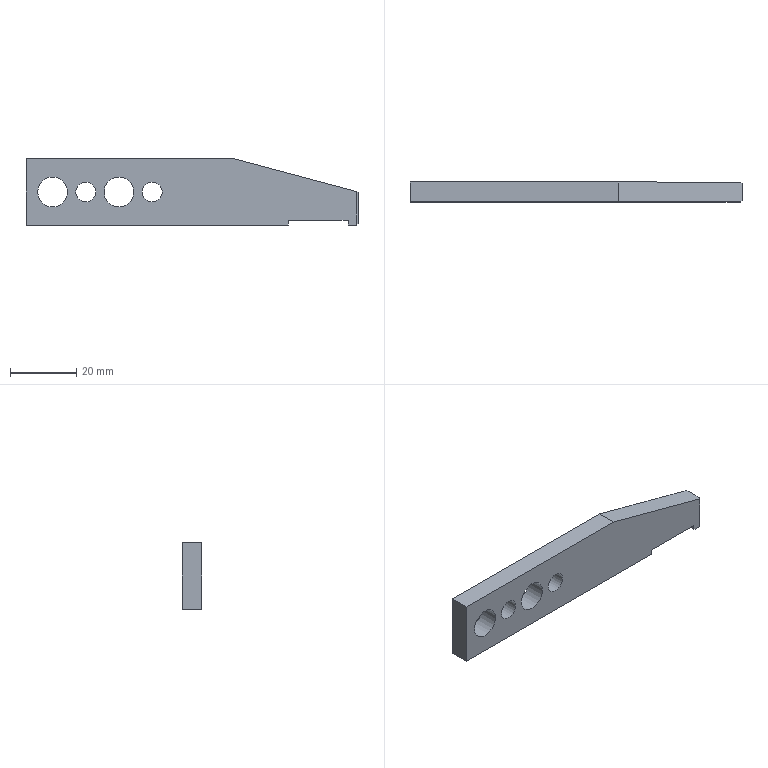Part | NX | features BREP 1 | 1 solid | 18 faces | box 100 x 6 x 20 mm | volume 9606 mm3 | plane 12 | cylinder 6 | commonest cylinder face diameters 6 x2 9 x2 19 x2
STEP:
#1=CARTESIAN_POINT('',(-21.014,3.,0.));
#2=VERTEX_POINT('',#1);
#3=CARTESIAN_POINT('',(-100.,3.,0.));
#4=VERTEX_POINT('',#3);
#5=CARTESIAN_POINT('',(-100.,3.,0.));
#6=DIRECTION('',(-1.,0.,0.));
#7=VECTOR('',#6,1000.);
#8=LINE('',#5,#7);
#9=EDGE_CURVE('',#2,#4,#8,.T.);
#10=ORIENTED_EDGE('',*,*,#9,.F.);
#11=CARTESIAN_POINT('',(-21.014,-3.,0.));
#12=VERTEX_POINT('',#11);
#13=CARTESIAN_POINT('',(-12.,0.,0.));
#14=DIRECTION('',(0.,0.,-1.));
#15=DIRECTION('',(-1.,0.,0.));
#16=AXIS2_PLACEMENT_3D('',#13,#14,#15);
#17=CIRCLE('',#16,9.5);
#18=EDGE_CURVE('',#12,#2,#17,.T.);
#19=ORIENTED_EDGE('',*,*,#18,.F.);
#20=CARTESIAN_POINT('',(-100.,-3.,0.));
#21=VERTEX_POINT('',#20);
#22=CARTESIAN_POINT('',(-100.,-3.,0.));
#23=DIRECTION('',(-1.,0.,0.));
#24=VECTOR('',#23,1000.);
#25=LINE('',#22,#24);
#26=EDGE_CURVE('',#12,#21,#25,.T.);
#27=ORIENTED_EDGE('',*,*,#26,.T.);
#28=CARTESIAN_POINT('',(-100.,3.,0.));
#29=DIRECTION('',(0.,-1.,0.));
#30=VECTOR('',#29,1000.);
#31=LINE('',#28,#30);
#32=EDGE_CURVE('',#4,#21,#31,.T.);
#33=ORIENTED_EDGE('',*,*,#32,.F.);
#34=EDGE_LOOP('',(#10,#19,#27,#33));
#35=FACE_BOUND('',#34,.T.);
#36=CARTESIAN_POINT('',(-100.,3.,0.));
#37=DIRECTION('',(0.,0.,1.));
#38=DIRECTION('',(-1.,0.,0.));
#39=AXIS2_PLACEMENT_3D('',#36,#37,#38);
#40=PLANE('',#39);
#41=ADVANCED_FACE('',(#35),#40,.F.);
#42=CARTESIAN_POINT('',(-100.,-3.,20.));
#43=VERTEX_POINT('',#42);
#44=CARTESIAN_POINT('',(-100.,-3.,25.));
#45=DIRECTION('',(0.,0.,1.));
#46=VECTOR('',#45,1000.);
#47=LINE('',#44,#46);
#48=EDGE_CURVE('',#21,#43,#47,.T.);
#49=ORIENTED_EDGE('',*,*,#48,.T.);
#50=CARTESIAN_POINT('',(-100.,3.,20.));
#51=VERTEX_POINT('',#50);
#52=CARTESIAN_POINT('',(-100.,-65.879,20.));
#53=DIRECTION('',(0.,1.,0.));
#54=VECTOR('',#53,1000.);
#55=LINE('',#52,#54);
#56=EDGE_CURVE('',#43,#51,#55,.T.);
#57=ORIENTED_EDGE('',*,*,#56,.T.);
#58=CARTESIAN_POINT('',(-100.,3.,25.));
#59=DIRECTION('',(0.,0.,1.));
#60=VECTOR('',#59,1000.);
#61=LINE('',#58,#60);
#62=EDGE_CURVE('',#4,#51,#61,.T.);
#63=ORIENTED_EDGE('',*,*,#62,.F.);
#64=ORIENTED_EDGE('',*,*,#32,.T.);
#65=EDGE_LOOP('',(#49,#57,#63,#64));
#66=FACE_BOUND('',#65,.T.);
#67=CARTESIAN_POINT('',(-100.,3.,25.));
#68=DIRECTION('',(1.,0.,0.));
#69=DIRECTION('',(0.,0.,1.));
#70=AXIS2_PLACEMENT_3D('',#67,#68,#69);
#71=PLANE('',#70);
#72=ADVANCED_FACE('',(#66),#71,.F.);
#73=CARTESIAN_POINT('',(-37.321,3.,20.));
#74=VERTEX_POINT('',#73);
#75=CARTESIAN_POINT('',(-0.5,3.,10.134));
#76=VERTEX_POINT('',#75);
#77=CARTESIAN_POINT('',(0.,3.,10.));
#78=DIRECTION('',(0.9659,0.,-0.2588));
#79=VECTOR('',#78,1000.);
#80=LINE('',#77,#79);
#81=EDGE_CURVE('',#74,#76,#80,.T.);
#82=ORIENTED_EDGE('',*,*,#81,.F.);
#83=CARTESIAN_POINT('',(-37.321,-3.,20.));
#84=VERTEX_POINT('',#83);
#85=CARTESIAN_POINT('',(-37.321,-65.879,20.));
#86=DIRECTION('',(0.,1.,0.));
#87=VECTOR('',#86,1000.);
#88=LINE('',#85,#87);
#89=EDGE_CURVE('',#84,#74,#88,.T.);
#90=ORIENTED_EDGE('',*,*,#89,.F.);
#91=CARTESIAN_POINT('',(-0.5,-3.,10.134));
#92=VERTEX_POINT('',#91);
#93=CARTESIAN_POINT('',(0.,-3.,10.));
#94=DIRECTION('',(0.9659,0.,-0.2588));
#95=VECTOR('',#94,1000.);
#96=LINE('',#93,#95);
#97=EDGE_CURVE('',#84,#92,#96,.T.);
#98=ORIENTED_EDGE('',*,*,#97,.T.);
#99=CARTESIAN_POINT('',(0.,-2.5,10.));
#100=VERTEX_POINT('',#99);
#101=CARTESIAN_POINT('',(1.293,-1.207,9.653));
#102=DIRECTION('',(0.6947,0.6947,-0.1862));
#103=VECTOR('',#102,1000.);
#104=LINE('',#101,#103);
#105=EDGE_CURVE('',#92,#100,#104,.T.);
#106=ORIENTED_EDGE('',*,*,#105,.T.);
#107=CARTESIAN_POINT('',(0.,2.5,10.));
#108=VERTEX_POINT('',#107);
#109=CARTESIAN_POINT('',(0.,3.,10.));
#110=DIRECTION('',(0.,-1.,0.));
#111=VECTOR('',#110,1000.);
#112=LINE('',#109,#111);
#113=EDGE_CURVE('',#108,#100,#112,.T.);
#114=ORIENTED_EDGE('',*,*,#113,.F.);
#115=CARTESIAN_POINT('',(0.8106,1.689,9.783));
#116=DIRECTION('',(-0.6947,0.6947,0.1862));
#117=VECTOR('',#116,1000.);
#118=LINE('',#115,#117);
#119=EDGE_CURVE('',#108,#76,#118,.T.);
#120=ORIENTED_EDGE('',*,*,#119,.T.);
#121=EDGE_LOOP('',(#82,#90,#98,#106,#114,#120));
#122=FACE_BOUND('',#121,.T.);
#123=CARTESIAN_POINT('',(0.,3.,10.));
#124=DIRECTION('',(-0.2588,0.,-0.9659));
#125=DIRECTION('',(0.9659,0.,-0.2588));
#126=AXIS2_PLACEMENT_3D('',#123,#124,#125);
#127=PLANE('',#126);
#128=ADVANCED_FACE('',(#122),#127,.F.);
#129=ORIENTED_EDGE('',*,*,#113,.T.);
#130=CARTESIAN_POINT('',(0.,-2.5,0.5));
#131=VERTEX_POINT('',#130);
#132=CARTESIAN_POINT('',(0.,-2.5,0.5));
#133=DIRECTION('',(0.,0.,-1.));
#134=VECTOR('',#133,1000.);
#135=LINE('',#132,#134);
#136=EDGE_CURVE('',#100,#131,#135,.T.);
#137=ORIENTED_EDGE('',*,*,#136,.T.);
#138=CARTESIAN_POINT('',(0.,2.5,0.5));
#139=VERTEX_POINT('',#138);
#140=CARTESIAN_POINT('',(0.,3.,0.5));
#141=DIRECTION('',(0.,1.,0.));
#142=VECTOR('',#141,1000.);
#143=LINE('',#140,#142);
#144=EDGE_CURVE('',#131,#139,#143,.T.);
#145=ORIENTED_EDGE('',*,*,#144,.T.);
#146=CARTESIAN_POINT('',(0.,2.5,0.));
#147=DIRECTION('',(0.,0.,1.));
#148=VECTOR('',#147,1000.);
#149=LINE('',#146,#148);
#150=EDGE_CURVE('',#139,#108,#149,.T.);
#151=ORIENTED_EDGE('',*,*,#150,.T.);
#152=EDGE_LOOP('',(#129,#137,#145,#151));
#153=FACE_BOUND('',#152,.T.);
#154=CARTESIAN_POINT('',(0.,3.,0.));
#155=DIRECTION('',(-1.,0.,0.));
#156=DIRECTION('',(0.,0.,-1.));
#157=AXIS2_PLACEMENT_3D('',#154,#155,#156);
#158=PLANE('',#157);
#159=ADVANCED_FACE('',(#153),#158,.F.);
#160=CARTESIAN_POINT('',(-0.5,3.,0.));
#161=VERTEX_POINT('',#160);
#162=CARTESIAN_POINT('',(-2.986,3.,0.));
#163=VERTEX_POINT('',#162);
#164=CARTESIAN_POINT('',(-100.,3.,0.));
#165=DIRECTION('',(-1.,0.,0.));
#166=VECTOR('',#165,1000.);
#167=LINE('',#164,#166);
#168=EDGE_CURVE('',#161,#163,#167,.T.);
#169=ORIENTED_EDGE('',*,*,#168,.F.);
#170=CARTESIAN_POINT('',(-0.5,-3.,0.));
#171=VERTEX_POINT('',#170);
#172=CARTESIAN_POINT('',(-0.5,3.,0.));
#173=DIRECTION('',(0.,-1.,0.));
#174=VECTOR('',#173,1000.);
#175=LINE('',#172,#174);
#176=EDGE_CURVE('',#161,#171,#175,.T.);
#177=ORIENTED_EDGE('',*,*,#176,.T.);
#178=CARTESIAN_POINT('',(-2.986,-3.,0.));
#179=VERTEX_POINT('',#178);
#180=CARTESIAN_POINT('',(-100.,-3.,0.));
#181=DIRECTION('',(-1.,0.,0.));
#182=VECTOR('',#181,1000.);
#183=LINE('',#180,#182);
#184=EDGE_CURVE('',#171,#179,#183,.T.);
#185=ORIENTED_EDGE('',*,*,#184,.T.);
#186=CARTESIAN_POINT('',(-12.,0.,0.));
#187=DIRECTION('',(0.,0.,-1.));
#188=DIRECTION('',(-1.,0.,0.));
#189=AXIS2_PLACEMENT_3D('',#186,#187,#188);
#190=CIRCLE('',#189,9.5);
#191=EDGE_CURVE('',#163,#179,#190,.T.);
#192=ORIENTED_EDGE('',*,*,#191,.F.);
#193=EDGE_LOOP('',(#169,#177,#185,#192));
#194=FACE_BOUND('',#193,.T.);
#195=CARTESIAN_POINT('',(-100.,3.,0.));
#196=DIRECTION('',(0.,0.,1.));
#197=DIRECTION('',(-1.,0.,0.));
#198=AXIS2_PLACEMENT_3D('',#195,#196,#197);
#199=PLANE('',#198);
#200=ADVANCED_FACE('',(#194),#199,.F.);
#201=CARTESIAN_POINT('',(-72.,3.,14.5));
#202=VERTEX_POINT('',#201);
#203=CARTESIAN_POINT('',(-72.,3.,10.));
#204=DIRECTION('',(0.,1.,0.));
#205=DIRECTION('',(0.,0.,1.));
#206=AXIS2_PLACEMENT_3D('',#203,#204,#205);
#207=CIRCLE('',#206,4.5);
#208=EDGE_CURVE('',#202,#202,#207,.T.);
#209=ORIENTED_EDGE('',*,*,#208,.F.);
#210=EDGE_LOOP('',(#209));
#211=FACE_BOUND('',#210,.T.);
#212=CARTESIAN_POINT('',(-92.,3.,14.5));
#213=VERTEX_POINT('',#212);
#214=CARTESIAN_POINT('',(-92.,3.,10.));
#215=DIRECTION('',(0.,1.,0.));
#216=DIRECTION('',(0.,0.,1.));
#217=AXIS2_PLACEMENT_3D('',#214,#215,#216);
#218=CIRCLE('',#217,4.5);
#219=EDGE_CURVE('',#213,#213,#218,.T.);
#220=ORIENTED_EDGE('',*,*,#219,.F.);
#221=EDGE_LOOP('',(#220));
#222=FACE_BOUND('',#221,.T.);
#223=CARTESIAN_POINT('',(-82.,3.,13.));
#224=VERTEX_POINT('',#223);
#225=CARTESIAN_POINT('',(-82.,3.,10.));
#226=DIRECTION('',(0.,1.,0.));
#227=DIRECTION('',(0.,0.,1.));
#228=AXIS2_PLACEMENT_3D('',#225,#226,#227);
#229=CIRCLE('',#228,3.);
#230=EDGE_CURVE('',#224,#224,#229,.T.);
#231=ORIENTED_EDGE('',*,*,#230,.F.);
#232=EDGE_LOOP('',(#231));
#233=FACE_BOUND('',#232,.T.);
#234=CARTESIAN_POINT('',(-62.,3.,13.));
#235=VERTEX_POINT('',#234);
#236=CARTESIAN_POINT('',(-62.,3.,10.));
#237=DIRECTION('',(0.,1.,0.));
#238=DIRECTION('',(0.,0.,1.));
#239=AXIS2_PLACEMENT_3D('',#236,#237,#238);
#240=CIRCLE('',#239,3.);
#241=EDGE_CURVE('',#235,#235,#240,.T.);
#242=ORIENTED_EDGE('',*,*,#241,.F.);
#243=EDGE_LOOP('',(#242));
#244=FACE_BOUND('',#243,.T.);
#245=ORIENTED_EDGE('',*,*,#62,.T.);
#246=CARTESIAN_POINT('',(-100.,3.,20.));
#247=DIRECTION('',(-1.,0.,0.));
#248=VECTOR('',#247,1000.);
#249=LINE('',#246,#248);
#250=EDGE_CURVE('',#74,#51,#249,.T.);
#251=ORIENTED_EDGE('',*,*,#250,.F.);
#252=ORIENTED_EDGE('',*,*,#81,.T.);
#253=CARTESIAN_POINT('',(-0.5,3.,0.));
#254=DIRECTION('',(0.,0.,-1.));
#255=VECTOR('',#254,1000.);
#256=LINE('',#253,#255);
#257=EDGE_CURVE('',#76,#161,#256,.T.);
#258=ORIENTED_EDGE('',*,*,#257,.T.);
#259=ORIENTED_EDGE('',*,*,#168,.T.);
#260=CARTESIAN_POINT('',(-2.986,3.,1.5));
#261=VERTEX_POINT('',#260);
#262=CARTESIAN_POINT('',(-2.986,3.,1.5));
#263=DIRECTION('',(0.,0.,1.));
#264=VECTOR('',#263,1000.);
#265=LINE('',#262,#264);
#266=EDGE_CURVE('',#163,#261,#265,.T.);
#267=ORIENTED_EDGE('',*,*,#266,.T.);
#268=CARTESIAN_POINT('',(-21.014,3.,1.5));
#269=VERTEX_POINT('',#268);
#270=CARTESIAN_POINT('',(0.,3.,1.5));
#271=DIRECTION('',(1.,0.,0.));
#272=VECTOR('',#271,1000.);
#273=LINE('',#270,#272);
#274=EDGE_CURVE('',#269,#261,#273,.T.);
#275=ORIENTED_EDGE('',*,*,#274,.F.);
#276=CARTESIAN_POINT('',(-21.014,3.,1.5));
#277=DIRECTION('',(0.,0.,-1.));
#278=VECTOR('',#277,1000.);
#279=LINE('',#276,#278);
#280=EDGE_CURVE('',#269,#2,#279,.T.);
#281=ORIENTED_EDGE('',*,*,#280,.T.);
#282=ORIENTED_EDGE('',*,*,#9,.T.);
#283=EDGE_LOOP('',(#245,#251,#252,#258,#259,#267,#275,#281,#282));
#284=FACE_BOUND('',#283,.T.);
#285=CARTESIAN_POINT('',(0.,3.,0.));
#286=DIRECTION('',(0.,-1.,0.));
#287=DIRECTION('',(0.,0.,1.));
#288=AXIS2_PLACEMENT_3D('',#285,#286,#287);
#289=PLANE('',#288);
#290=ADVANCED_FACE('',(#211,#222,#233,#244,#284),#289,.F.);
#291=CARTESIAN_POINT('',(-100.,-3.,20.));
#292=DIRECTION('',(-1.,0.,0.));
#293=VECTOR('',#292,1000.);
#294=LINE('',#291,#293);
#295=EDGE_CURVE('',#84,#43,#294,.T.);
#296=ORIENTED_EDGE('',*,*,#295,.T.);
#297=ORIENTED_EDGE('',*,*,#48,.F.);
#298=ORIENTED_EDGE('',*,*,#26,.F.);
#299=CARTESIAN_POINT('',(-21.014,-3.,1.5));
#300=VERTEX_POINT('',#299);
#301=CARTESIAN_POINT('',(-21.014,-3.,1.5));
#302=DIRECTION('',(0.,0.,-1.));
#303=VECTOR('',#302,1000.);
#304=LINE('',#301,#303);
#305=EDGE_CURVE('',#300,#12,#304,.T.);
#306=ORIENTED_EDGE('',*,*,#305,.F.);
#307=CARTESIAN_POINT('',(-2.986,-3.,1.5));
#308=VERTEX_POINT('',#307);
#309=CARTESIAN_POINT('',(0.,-3.,1.5));
#310=DIRECTION('',(1.,0.,0.));
#311=VECTOR('',#310,1000.);
#312=LINE('',#309,#311);
#313=EDGE_CURVE('',#300,#308,#312,.T.);
#314=ORIENTED_EDGE('',*,*,#313,.T.);
#315=CARTESIAN_POINT('',(-2.986,-3.,1.5));
#316=DIRECTION('',(0.,0.,1.));
#317=VECTOR('',#316,1000.);
#318=LINE('',#315,#317);
#319=EDGE_CURVE('',#179,#308,#318,.T.);
#320=ORIENTED_EDGE('',*,*,#319,.F.);
#321=ORIENTED_EDGE('',*,*,#184,.F.);
#322=CARTESIAN_POINT('',(-0.5,-3.,10.));
#323=DIRECTION('',(0.,0.,1.));
#324=VECTOR('',#323,1000.);
#325=LINE('',#322,#324);
#326=EDGE_CURVE('',#171,#92,#325,.T.);
#327=ORIENTED_EDGE('',*,*,#326,.T.);
#328=ORIENTED_EDGE('',*,*,#97,.F.);
#329=EDGE_LOOP('',(#296,#297,#298,#306,#314,#320,#321,#327,#328));
#330=FACE_BOUND('',#329,.T.);
#331=CARTESIAN_POINT('',(-72.,-3.,14.5));
#332=VERTEX_POINT('',#331);
#333=CARTESIAN_POINT('',(-72.,-3.,10.));
#334=DIRECTION('',(0.,1.,0.));
#335=DIRECTION('',(0.,0.,1.));
#336=AXIS2_PLACEMENT_3D('',#333,#334,#335);
#337=CIRCLE('',#336,4.5);
#338=EDGE_CURVE('',#332,#332,#337,.T.);
#339=ORIENTED_EDGE('',*,*,#338,.T.);
#340=EDGE_LOOP('',(#339));
#341=FACE_BOUND('',#340,.T.);
#342=CARTESIAN_POINT('',(-92.,-3.,14.5));
#343=VERTEX_POINT('',#342);
#344=CARTESIAN_POINT('',(-92.,-3.,10.));
#345=DIRECTION('',(0.,1.,0.));
#346=DIRECTION('',(0.,0.,1.));
#347=AXIS2_PLACEMENT_3D('',#344,#345,#346);
#348=CIRCLE('',#347,4.5);
#349=EDGE_CURVE('',#343,#343,#348,.T.);
#350=ORIENTED_EDGE('',*,*,#349,.T.);
#351=EDGE_LOOP('',(#350));
#352=FACE_BOUND('',#351,.T.);
#353=CARTESIAN_POINT('',(-82.,-3.,13.));
#354=VERTEX_POINT('',#353);
#355=CARTESIAN_POINT('',(-82.,-3.,10.));
#356=DIRECTION('',(0.,1.,0.));
#357=DIRECTION('',(0.,0.,1.));
#358=AXIS2_PLACEMENT_3D('',#355,#356,#357);
#359=CIRCLE('',#358,3.);
#360=EDGE_CURVE('',#354,#354,#359,.T.);
#361=ORIENTED_EDGE('',*,*,#360,.T.);
#362=EDGE_LOOP('',(#361));
#363=FACE_BOUND('',#362,.T.);
#364=CARTESIAN_POINT('',(-62.,-3.,13.));
#365=VERTEX_POINT('',#364);
#366=CARTESIAN_POINT('',(-62.,-3.,10.));
#367=DIRECTION('',(0.,1.,0.));
#368=DIRECTION('',(0.,0.,1.));
#369=AXIS2_PLACEMENT_3D('',#366,#367,#368);
#370=CIRCLE('',#369,3.);
#371=EDGE_CURVE('',#365,#365,#370,.T.);
#372=ORIENTED_EDGE('',*,*,#371,.T.);
#373=EDGE_LOOP('',(#372));
#374=FACE_BOUND('',#373,.T.);
#375=CARTESIAN_POINT('',(0.,-3.,0.));
#376=DIRECTION('',(0.,-1.,0.));
#377=DIRECTION('',(0.,0.,1.));
#378=AXIS2_PLACEMENT_3D('',#375,#376,#377);
#379=PLANE('',#378);
#380=ADVANCED_FACE('',(#330,#341,#352,#363,#374),#379,.T.);
#381=CARTESIAN_POINT('',(-12.,0.,1.5));
#382=DIRECTION('',(0.,0.,-1.));
#383=DIRECTION('',(-1.,0.,0.));
#384=AXIS2_PLACEMENT_3D('',#381,#382,#383);
#385=CIRCLE('',#384,9.5);
#386=EDGE_CURVE('',#300,#269,#385,.T.);
#387=ORIENTED_EDGE('',*,*,#386,.F.);
#388=ORIENTED_EDGE('',*,*,#305,.T.);
#389=ORIENTED_EDGE('',*,*,#18,.T.);
#390=ORIENTED_EDGE('',*,*,#280,.F.);
#391=EDGE_LOOP('',(#387,#388,#389,#390));
#392=FACE_BOUND('',#391,.T.);
#393=CARTESIAN_POINT('',(-12.,0.,1.5));
#394=DIRECTION('',(0.,0.,-1.));
#395=DIRECTION('',(1.,0.,0.));
#396=AXIS2_PLACEMENT_3D('',#393,#394,#395);
#397=CYLINDRICAL_SURFACE('',#396,9.5);
#398=ADVANCED_FACE('',(#392),#397,.F.);
#399=ORIENTED_EDGE('',*,*,#191,.T.);
#400=ORIENTED_EDGE('',*,*,#319,.T.);
#401=CARTESIAN_POINT('',(-12.,0.,1.5));
#402=DIRECTION('',(0.,0.,-1.));
#403=DIRECTION('',(-1.,0.,0.));
#404=AXIS2_PLACEMENT_3D('',#401,#402,#403);
#405=CIRCLE('',#404,9.5);
#406=EDGE_CURVE('',#261,#308,#405,.T.);
#407=ORIENTED_EDGE('',*,*,#406,.F.);
#408=ORIENTED_EDGE('',*,*,#266,.F.);
#409=EDGE_LOOP('',(#399,#400,#407,#408));
#410=FACE_BOUND('',#409,.T.);
#411=CARTESIAN_POINT('',(-12.,0.,1.5));
#412=DIRECTION('',(0.,0.,-1.));
#413=DIRECTION('',(1.,0.,0.));
#414=AXIS2_PLACEMENT_3D('',#411,#412,#413);
#415=CYLINDRICAL_SURFACE('',#414,9.5);
#416=ADVANCED_FACE('',(#410),#415,.F.);
#417=ORIENTED_EDGE('',*,*,#274,.T.);
#418=ORIENTED_EDGE('',*,*,#406,.T.);
#419=ORIENTED_EDGE('',*,*,#313,.F.);
#420=ORIENTED_EDGE('',*,*,#386,.T.);
#421=EDGE_LOOP('',(#417,#418,#419,#420));
#422=FACE_BOUND('',#421,.T.);
#423=CARTESIAN_POINT('',(-12.,0.,1.5));
#424=DIRECTION('',(0.,0.,-1.));
#425=DIRECTION('',(1.,0.,0.));
#426=AXIS2_PLACEMENT_3D('',#423,#424,#425);
#427=PLANE('',#426);
#428=ADVANCED_FACE('',(#422),#427,.T.);
#429=ORIENTED_EDGE('',*,*,#371,.F.);
#430=EDGE_LOOP('',(#429));
#431=FACE_BOUND('',#430,.T.);
#432=ORIENTED_EDGE('',*,*,#241,.T.);
#433=EDGE_LOOP('',(#432));
#434=FACE_BOUND('',#433,.T.);
#435=CARTESIAN_POINT('',(-62.,3.,10.));
#436=DIRECTION('',(0.,1.,0.));
#437=DIRECTION('',(0.,0.,-1.));
#438=AXIS2_PLACEMENT_3D('',#435,#436,#437);
#439=CYLINDRICAL_SURFACE('',#438,3.);
#440=ADVANCED_FACE('',(#431,#434),#439,.F.);
#441=ORIENTED_EDGE('',*,*,#360,.F.);
#442=EDGE_LOOP('',(#441));
#443=FACE_BOUND('',#442,.T.);
#444=ORIENTED_EDGE('',*,*,#230,.T.);
#445=EDGE_LOOP('',(#444));
#446=FACE_BOUND('',#445,.T.);
#447=CARTESIAN_POINT('',(-82.,3.,10.));
#448=DIRECTION('',(0.,1.,0.));
#449=DIRECTION('',(0.,0.,-1.));
#450=AXIS2_PLACEMENT_3D('',#447,#448,#449);
#451=CYLINDRICAL_SURFACE('',#450,3.);
#452=ADVANCED_FACE('',(#443,#446),#451,.F.);
#453=ORIENTED_EDGE('',*,*,#349,.F.);
#454=EDGE_LOOP('',(#453));
#455=FACE_BOUND('',#454,.T.);
#456=ORIENTED_EDGE('',*,*,#219,.T.);
#457=EDGE_LOOP('',(#456));
#458=FACE_BOUND('',#457,.T.);
#459=CARTESIAN_POINT('',(-92.,3.,10.));
#460=DIRECTION('',(0.,1.,0.));
#461=DIRECTION('',(0.,0.,-1.));
#462=AXIS2_PLACEMENT_3D('',#459,#460,#461);
#463=CYLINDRICAL_SURFACE('',#462,4.5);
#464=ADVANCED_FACE('',(#455,#458),#463,.F.);
#465=ORIENTED_EDGE('',*,*,#338,.F.);
#466=EDGE_LOOP('',(#465));
#467=FACE_BOUND('',#466,.T.);
#468=ORIENTED_EDGE('',*,*,#208,.T.);
#469=EDGE_LOOP('',(#468));
#470=FACE_BOUND('',#469,.T.);
#471=CARTESIAN_POINT('',(-72.,3.,10.));
#472=DIRECTION('',(0.,1.,0.));
#473=DIRECTION('',(0.,0.,-1.));
#474=AXIS2_PLACEMENT_3D('',#471,#472,#473);
#475=CYLINDRICAL_SURFACE('',#474,4.5);
#476=ADVANCED_FACE('',(#467,#470),#475,.F.);
#477=ORIENTED_EDGE('',*,*,#144,.F.);
#478=CARTESIAN_POINT('',(1.5,-1.,2.));
#479=DIRECTION('',(-0.5774,-0.5774,-0.5774));
#480=VECTOR('',#479,1000.);
#481=LINE('',#478,#480);
#482=EDGE_CURVE('',#131,#171,#481,.T.);
#483=ORIENTED_EDGE('',*,*,#482,.T.);
#484=ORIENTED_EDGE('',*,*,#176,.F.);
#485=CARTESIAN_POINT('',(-0.5,3.,0.));
#486=DIRECTION('',(0.5774,-0.5774,0.5774));
#487=VECTOR('',#486,1000.);
#488=LINE('',#485,#487);
#489=EDGE_CURVE('',#161,#139,#488,.T.);
#490=ORIENTED_EDGE('',*,*,#489,.T.);
#491=EDGE_LOOP('',(#477,#483,#484,#490));
#492=FACE_BOUND('',#491,.T.);
#493=CARTESIAN_POINT('',(-0.5,3.,0.));
#494=DIRECTION('',(-0.7071,0.,0.7071));
#495=DIRECTION('',(0.,1.,0.));
#496=AXIS2_PLACEMENT_3D('',#493,#494,#495);
#497=PLANE('',#496);
#498=ADVANCED_FACE('',(#492),#497,.F.);
#499=ORIENTED_EDGE('',*,*,#105,.F.);
#500=ORIENTED_EDGE('',*,*,#326,.F.);
#501=ORIENTED_EDGE('',*,*,#482,.F.);
#502=ORIENTED_EDGE('',*,*,#136,.F.);
#503=EDGE_LOOP('',(#499,#500,#501,#502));
#504=FACE_BOUND('',#503,.T.);
#505=CARTESIAN_POINT('',(0.,-2.5,0.));
#506=DIRECTION('',(0.7071,-0.7071,0.));
#507=DIRECTION('',(0.,0.,-1.));
#508=AXIS2_PLACEMENT_3D('',#505,#506,#507);
#509=PLANE('',#508);
#510=ADVANCED_FACE('',(#504),#509,.T.);
#511=ORIENTED_EDGE('',*,*,#119,.F.);
#512=ORIENTED_EDGE('',*,*,#150,.F.);
#513=ORIENTED_EDGE('',*,*,#489,.F.);
#514=ORIENTED_EDGE('',*,*,#257,.F.);
#515=EDGE_LOOP('',(#511,#512,#513,#514));
#516=FACE_BOUND('',#515,.T.);
#517=CARTESIAN_POINT('',(-0.5,3.,0.));
#518=DIRECTION('',(-0.7071,-0.7071,0.));
#519=DIRECTION('',(0.,0.,1.));
#520=AXIS2_PLACEMENT_3D('',#517,#518,#519);
#521=PLANE('',#520);
#522=ADVANCED_FACE('',(#516),#521,.F.);
#523=ORIENTED_EDGE('',*,*,#89,.T.);
#524=ORIENTED_EDGE('',*,*,#250,.T.);
#525=ORIENTED_EDGE('',*,*,#56,.F.);
#526=ORIENTED_EDGE('',*,*,#295,.F.);
#527=EDGE_LOOP('',(#523,#524,#525,#526));
#528=FACE_BOUND('',#527,.T.);
#529=CARTESIAN_POINT('',(-100.,-65.879,20.));
#530=DIRECTION('',(0.,0.,-1.));
#531=DIRECTION('',(1.,0.,0.));
#532=AXIS2_PLACEMENT_3D('',#529,#530,#531);
#533=PLANE('',#532);
#534=ADVANCED_FACE('',(#528),#533,.F.);
#535=CLOSED_SHELL('',(#41,#72,#128,#159,#200,#290,#380,#398,#416,#428,#440,#452,#464,#476,#498,#510,#522,#534));
#536=MANIFOLD_SOLID_BREP('',#535);
#537=(LENGTH_UNIT()NAMED_UNIT(*)SI_UNIT(.MILLI.,.METRE.));
#538=UNCERTAINTY_MEASURE_WITH_UNIT(LENGTH_MEASURE(0.00001),#537,'','');
#539=(NAMED_UNIT(*)PLANE_ANGLE_UNIT()SI_UNIT($,.RADIAN.));
#540=(NAMED_UNIT(*)SI_UNIT($,.STERADIAN.)SOLID_ANGLE_UNIT());
#541=(GEOMETRIC_REPRESENTATION_CONTEXT(3)GLOBAL_UNCERTAINTY_ASSIGNED_CONTEXT((#538))GLOBAL_UNIT_ASSIGNED_CONTEXT((#537,#539,#540))REPRESENTATION_CONTEXT('',''));
#542=ADVANCED_BREP_SHAPE_REPRESENTATION('',(#536),#541);